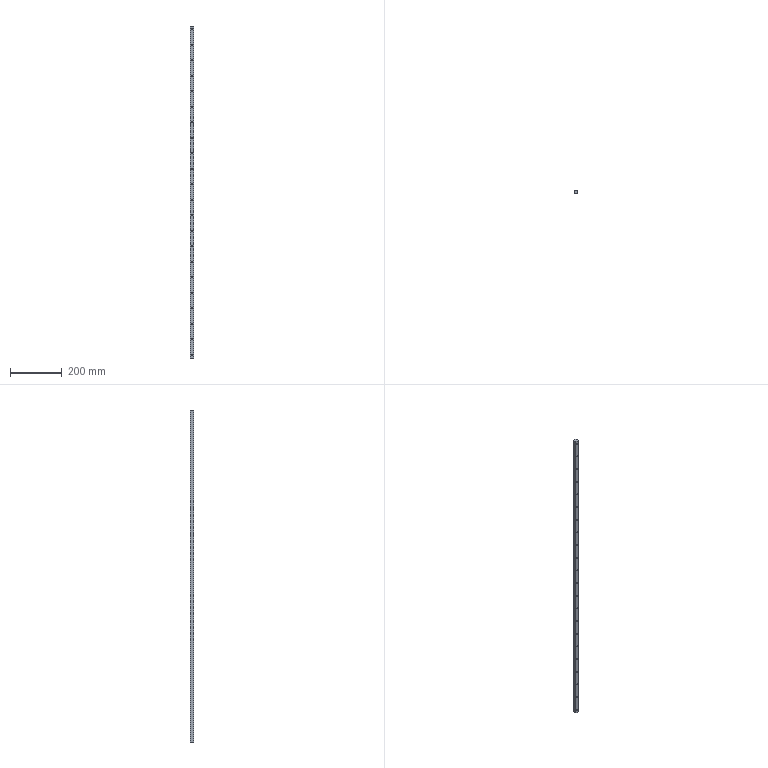Part | STEP file | SM140A-20-1140D-140A-600 Guide rail 600 | 1 solid | 116 faces | box 15 x 12.5 x 1284 mm | volume 233266 mm3 | cylinder 88 | plane 28 | commonest cylinder face diameters 4.5 x44 7.5 x44